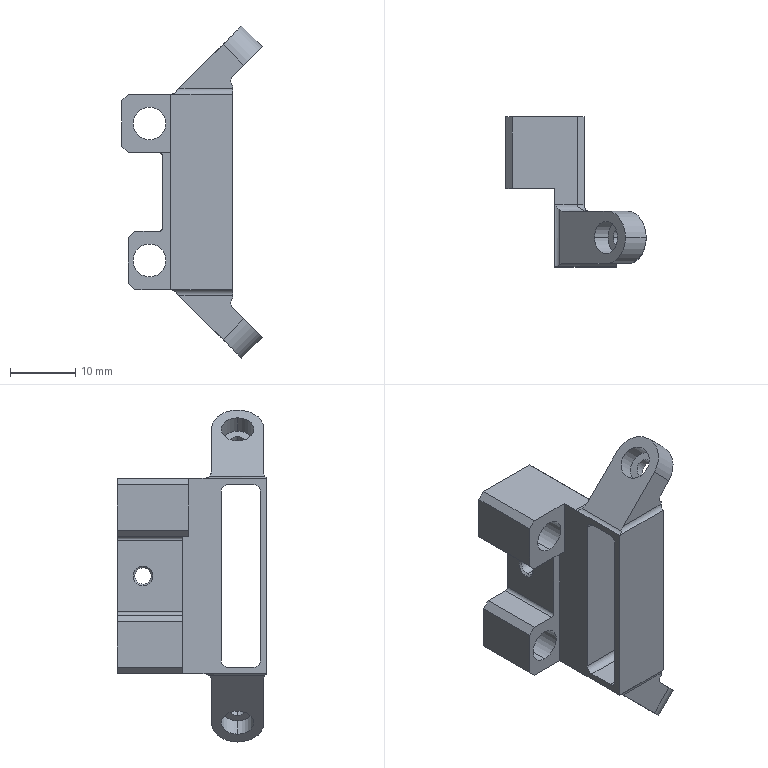CAM job | NX | 3+2 milling | part box 21.534 x 23 x 50.912 mm | stock box 26.622 x 26.466 x 57.912 mm
Tools:
number,name,description,diameter,corner_radius,flute_length,length,flutes
3,D3开粗,D3,3.0,0.0,9.0,50.0,2
1,D8开粗,D8,8.0,0.0,20.0,60.0,2
2,D6R1,圆鼻铣刀,6.0,1.0,18.0,50.0,2
Operations:
program,operation,operation_type,tool,method,geometry_group,spindle_rpm,surface_speed,feed_per_tooth,feed_cut,feed_plunge,cut_length_mm,path_length_mm,cut_time_min,machine_time_min
XX-CNC1,FLOOR_FACING,VolumeBased25DMillingOperation,D8开粗,METHOD,MCS_1,1061.0,100.0,0.1178,250.0,100.0,354.083,453.883,1.416,1.426
XX-CNC1,ADAPTIVE_MILLING,CavityMilling,D8开粗,METHOD,WORKPIECE,1061.0,100.0,0.1178,250.0,100.0,4259.672,6266.027,16.465,16.666
XX-CNC1,ADAPTIVE_MILLING_COPY,CavityMilling,D8开粗,METHOD,WORKPIECE,1061.0,100.0,0.1178,250.0,100.0,2479.805,7493.907,9.825,10.327
XX-CNC1,ADAPTIVE_MILLING_COPY_COPY,CavityMilling,D8开粗,METHOD,WORKPIECE,1061.0,100.0,0.1178,250.0,100.0,1148.598,7933.486,4.471,5.15
XX-CNC1,PLANAR_MILL_1,PlanarMilling,D6R1,METHOD,MCS_1,1061.0,100.0,0.1178,250.0,100.0,372.092,755.507,1.488,1.527
XX-CNC1,PLANAR_MILL_1_COPY,PlanarMilling,D6R1,METHOD,MCS_1,1061.0,100.0,0.1178,250.0,100.0,105.047,230.047,0.4202,0.4327
XX-CNC1,FLOOR_FACING_1_COPY,VolumeBased25DMillingOperation,D6R1,METHOD,WORKPIECE,1061.0,100.0,0.1178,250.0,100.0,145.398,251.932,0.5816,0.5922
XX-CNC1,FLOOR_FACING_1_COPY_COPY_COPY,VolumeBased25DMillingOperation,D6R1,METHOD,WORKPIECE,1061.0,100.0,0.1178,250.0,100.0,51.831,161.797,0.2073,0.2183
XX-CNC1,PLANAR_MILL_2,PlanarMilling,D6R1,METHOD,MCS_1,1061.0,100.0,0.1178,250.0,100.0,45.0,268.0,0.18,0.2023
XX-CNC1,FLOOR_FACING_1_COPY_COPY_COPY_COPY,VolumeBased25DMillingOperation,D3开粗,METHOD,WORKPIECE,1061.0,100.0,0.1178,250.0,100.0,206.25,318.816,0.825,0.8363
XX-CNC1,PLANAR_MILL_3,PlanarMilling,D3开粗,METHOD,MCS_1,1061.0,100.0,0.1178,250.0,100.0,42.432,149.432,0.1697,0.1804
XX-CNC1,PLANAR_MILL,PlanarMilling,D3开粗,METHOD,MCS_1,1061.0,100.0,0.1178,250.0,100.0,1374.82,1483.32,5.499,5.51